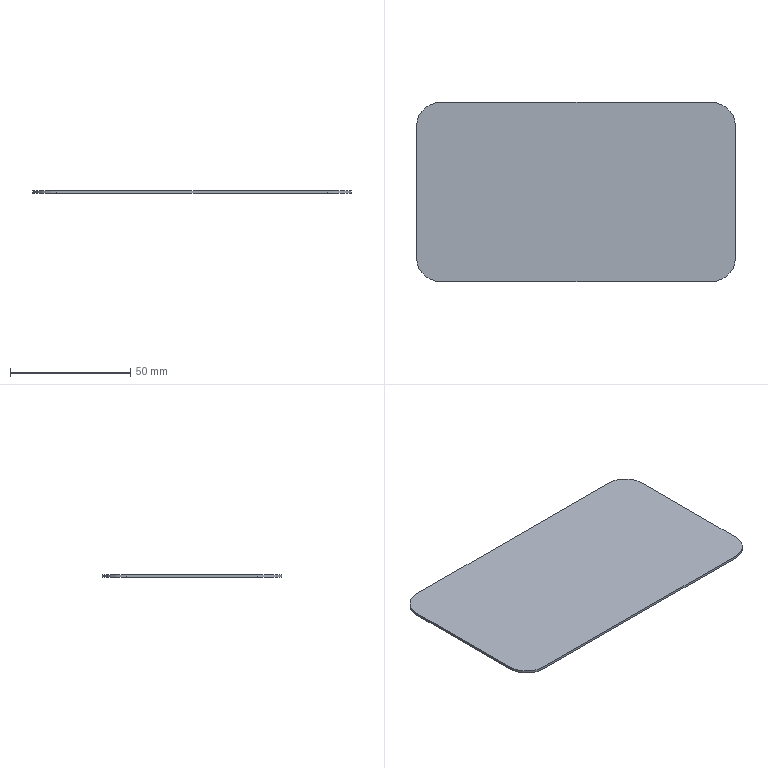Part | SolidWorks | features Extrusion 1, Fillet 1 | 1 solid | 10 faces | box 132.8 x 74.7 x 1 mm | volume 9834 mm3 | plane 6 | cylinder 4 | commonest cylinder face diameters 20 x4
STEP:
#1=CARTESIAN_POINT('',(-66.4,-27.35,1.));
#2=VERTEX_POINT('',#1);
#3=CARTESIAN_POINT('',(-66.4,27.35,1.));
#4=VERTEX_POINT('',#3);
#5=CARTESIAN_POINT('',(-66.4,-37.35,1.));
#6=DIRECTION('',(0.,1.,0.));
#7=VECTOR('',#6,1000.);
#8=LINE('',#5,#7);
#9=EDGE_CURVE('',#2,#4,#8,.T.);
#10=ORIENTED_EDGE('',*,*,#9,.T.);
#11=CARTESIAN_POINT('',(-66.4,27.35,0.));
#12=VERTEX_POINT('',#11);
#13=CARTESIAN_POINT('',(-66.4,27.35,1.));
#14=DIRECTION('',(0.,0.,-1.));
#15=VECTOR('',#14,1000.);
#16=LINE('',#13,#15);
#17=EDGE_CURVE('',#4,#12,#16,.T.);
#18=ORIENTED_EDGE('',*,*,#17,.T.);
#19=CARTESIAN_POINT('',(-66.4,-27.35,0.));
#20=VERTEX_POINT('',#19);
#21=CARTESIAN_POINT('',(-66.4,-37.35,0.));
#22=DIRECTION('',(0.,1.,0.));
#23=VECTOR('',#22,1000.);
#24=LINE('',#21,#23);
#25=EDGE_CURVE('',#20,#12,#24,.T.);
#26=ORIENTED_EDGE('',*,*,#25,.F.);
#27=CARTESIAN_POINT('',(-66.4,-27.35,1.));
#28=DIRECTION('',(0.,0.,1.));
#29=VECTOR('',#28,1000.);
#30=LINE('',#27,#29);
#31=EDGE_CURVE('',#20,#2,#30,.T.);
#32=ORIENTED_EDGE('',*,*,#31,.T.);
#33=EDGE_LOOP('',(#10,#18,#26,#32));
#34=FACE_OUTER_BOUND('',#33,.T.);
#35=CARTESIAN_POINT('',(-66.4,-37.35,1.));
#36=DIRECTION('',(-1.,0.,0.));
#37=DIRECTION('',(0.,0.,1.));
#38=AXIS2_PLACEMENT_3D('',#35,#36,#37);
#39=PLANE('',#38);
#40=ADVANCED_FACE('',(#34),#39,.T.);
#41=CARTESIAN_POINT('',(-56.4,-37.35,0.));
#42=VERTEX_POINT('',#41);
#43=CARTESIAN_POINT('',(56.4,-37.35,0.));
#44=VERTEX_POINT('',#43);
#45=CARTESIAN_POINT('',(-66.4,-37.35,0.));
#46=DIRECTION('',(1.,0.,0.));
#47=VECTOR('',#46,1000.);
#48=LINE('',#45,#47);
#49=EDGE_CURVE('',#42,#44,#48,.T.);
#50=ORIENTED_EDGE('',*,*,#49,.T.);
#51=CARTESIAN_POINT('',(56.4,-37.35,1.));
#52=VERTEX_POINT('',#51);
#53=CARTESIAN_POINT('',(56.4,-37.35,1.));
#54=DIRECTION('',(0.,0.,1.));
#55=VECTOR('',#54,1000.);
#56=LINE('',#53,#55);
#57=EDGE_CURVE('',#44,#52,#56,.T.);
#58=ORIENTED_EDGE('',*,*,#57,.T.);
#59=CARTESIAN_POINT('',(-56.4,-37.35,1.));
#60=VERTEX_POINT('',#59);
#61=CARTESIAN_POINT('',(-66.4,-37.35,1.));
#62=DIRECTION('',(1.,0.,0.));
#63=VECTOR('',#62,1000.);
#64=LINE('',#61,#63);
#65=EDGE_CURVE('',#60,#52,#64,.T.);
#66=ORIENTED_EDGE('',*,*,#65,.F.);
#67=CARTESIAN_POINT('',(-56.4,-37.35,0.));
#68=DIRECTION('',(0.,0.,-1.));
#69=VECTOR('',#68,1000.);
#70=LINE('',#67,#69);
#71=EDGE_CURVE('',#60,#42,#70,.T.);
#72=ORIENTED_EDGE('',*,*,#71,.T.);
#73=EDGE_LOOP('',(#50,#58,#66,#72));
#74=FACE_OUTER_BOUND('',#73,.T.);
#75=CARTESIAN_POINT('',(-66.4,-37.35,1.));
#76=DIRECTION('',(0.,1.,0.));
#77=DIRECTION('',(0.,0.,1.));
#78=AXIS2_PLACEMENT_3D('',#75,#76,#77);
#79=PLANE('',#78);
#80=ADVANCED_FACE('',(#74),#79,.F.);
#81=CARTESIAN_POINT('',(66.4,-27.35,0.));
#82=VERTEX_POINT('',#81);
#83=CARTESIAN_POINT('',(66.4,27.35,0.));
#84=VERTEX_POINT('',#83);
#85=CARTESIAN_POINT('',(66.4,-37.35,0.));
#86=DIRECTION('',(0.,1.,0.));
#87=VECTOR('',#86,1000.);
#88=LINE('',#85,#87);
#89=EDGE_CURVE('',#82,#84,#88,.T.);
#90=ORIENTED_EDGE('',*,*,#89,.T.);
#91=CARTESIAN_POINT('',(66.4,27.35,1.));
#92=VERTEX_POINT('',#91);
#93=CARTESIAN_POINT('',(66.4,27.35,1.));
#94=DIRECTION('',(0.,0.,1.));
#95=VECTOR('',#94,1000.);
#96=LINE('',#93,#95);
#97=EDGE_CURVE('',#84,#92,#96,.T.);
#98=ORIENTED_EDGE('',*,*,#97,.T.);
#99=CARTESIAN_POINT('',(66.4,-27.35,1.));
#100=VERTEX_POINT('',#99);
#101=CARTESIAN_POINT('',(66.4,-37.35,1.));
#102=DIRECTION('',(0.,1.,0.));
#103=VECTOR('',#102,1000.);
#104=LINE('',#101,#103);
#105=EDGE_CURVE('',#100,#92,#104,.T.);
#106=ORIENTED_EDGE('',*,*,#105,.F.);
#107=CARTESIAN_POINT('',(66.4,-27.35,1.));
#108=DIRECTION('',(0.,0.,-1.));
#109=VECTOR('',#108,1000.);
#110=LINE('',#107,#109);
#111=EDGE_CURVE('',#100,#82,#110,.T.);
#112=ORIENTED_EDGE('',*,*,#111,.T.);
#113=EDGE_LOOP('',(#90,#98,#106,#112));
#114=FACE_OUTER_BOUND('',#113,.T.);
#115=CARTESIAN_POINT('',(66.4,-37.35,1.));
#116=DIRECTION('',(-1.,0.,0.));
#117=DIRECTION('',(0.,0.,1.));
#118=AXIS2_PLACEMENT_3D('',#115,#116,#117);
#119=PLANE('',#118);
#120=ADVANCED_FACE('',(#114),#119,.F.);
#121=CARTESIAN_POINT('',(-56.4,37.35,1.));
#122=VERTEX_POINT('',#121);
#123=CARTESIAN_POINT('',(56.4,37.35,1.));
#124=VERTEX_POINT('',#123);
#125=CARTESIAN_POINT('',(-66.4,37.35,1.));
#126=DIRECTION('',(1.,0.,0.));
#127=VECTOR('',#126,1000.);
#128=LINE('',#125,#127);
#129=EDGE_CURVE('',#122,#124,#128,.T.);
#130=ORIENTED_EDGE('',*,*,#129,.T.);
#131=CARTESIAN_POINT('',(56.4,37.35,0.));
#132=VERTEX_POINT('',#131);
#133=CARTESIAN_POINT('',(56.4,37.35,0.));
#134=DIRECTION('',(0.,0.,-1.));
#135=VECTOR('',#134,1000.);
#136=LINE('',#133,#135);
#137=EDGE_CURVE('',#124,#132,#136,.T.);
#138=ORIENTED_EDGE('',*,*,#137,.T.);
#139=CARTESIAN_POINT('',(-56.4,37.35,0.));
#140=VERTEX_POINT('',#139);
#141=CARTESIAN_POINT('',(-66.4,37.35,0.));
#142=DIRECTION('',(1.,0.,0.));
#143=VECTOR('',#142,1000.);
#144=LINE('',#141,#143);
#145=EDGE_CURVE('',#140,#132,#144,.T.);
#146=ORIENTED_EDGE('',*,*,#145,.F.);
#147=CARTESIAN_POINT('',(-56.4,37.35,1.));
#148=DIRECTION('',(0.,0.,1.));
#149=VECTOR('',#148,1000.);
#150=LINE('',#147,#149);
#151=EDGE_CURVE('',#140,#122,#150,.T.);
#152=ORIENTED_EDGE('',*,*,#151,.T.);
#153=EDGE_LOOP('',(#130,#138,#146,#152));
#154=FACE_OUTER_BOUND('',#153,.T.);
#155=CARTESIAN_POINT('',(-66.4,37.35,1.));
#156=DIRECTION('',(0.,1.,0.));
#157=DIRECTION('',(0.,0.,1.));
#158=AXIS2_PLACEMENT_3D('',#155,#156,#157);
#159=PLANE('',#158);
#160=ADVANCED_FACE('',(#154),#159,.T.);
#161=ORIENTED_EDGE('',*,*,#105,.T.);
#162=CARTESIAN_POINT('',(56.4,27.35,1.));
#163=DIRECTION('',(0.,0.,1.));
#164=DIRECTION('',(-1.,0.,0.));
#165=AXIS2_PLACEMENT_3D('',#162,#163,#164);
#166=CIRCLE('',#165,10.);
#167=EDGE_CURVE('',#92,#124,#166,.T.);
#168=ORIENTED_EDGE('',*,*,#167,.T.);
#169=ORIENTED_EDGE('',*,*,#129,.F.);
#170=CARTESIAN_POINT('',(-56.4,27.35,1.));
#171=DIRECTION('',(0.,0.,1.));
#172=DIRECTION('',(-1.,0.,0.));
#173=AXIS2_PLACEMENT_3D('',#170,#171,#172);
#174=CIRCLE('',#173,10.);
#175=EDGE_CURVE('',#122,#4,#174,.T.);
#176=ORIENTED_EDGE('',*,*,#175,.T.);
#177=ORIENTED_EDGE('',*,*,#9,.F.);
#178=CARTESIAN_POINT('',(-56.4,-27.35,1.));
#179=DIRECTION('',(0.,0.,1.));
#180=DIRECTION('',(-1.,0.,0.));
#181=AXIS2_PLACEMENT_3D('',#178,#179,#180);
#182=CIRCLE('',#181,10.);
#183=EDGE_CURVE('',#2,#60,#182,.T.);
#184=ORIENTED_EDGE('',*,*,#183,.T.);
#185=ORIENTED_EDGE('',*,*,#65,.T.);
#186=CARTESIAN_POINT('',(56.4,-27.35,1.));
#187=DIRECTION('',(0.,0.,1.));
#188=DIRECTION('',(-1.,0.,0.));
#189=AXIS2_PLACEMENT_3D('',#186,#187,#188);
#190=CIRCLE('',#189,10.);
#191=EDGE_CURVE('',#52,#100,#190,.T.);
#192=ORIENTED_EDGE('',*,*,#191,.T.);
#193=EDGE_LOOP('',(#161,#168,#169,#176,#177,#184,#185,#192));
#194=FACE_OUTER_BOUND('',#193,.T.);
#195=CARTESIAN_POINT('',(0.,0.,1.));
#196=DIRECTION('',(0.,0.,-1.));
#197=DIRECTION('',(-1.,0.,0.));
#198=AXIS2_PLACEMENT_3D('',#195,#196,#197);
#199=PLANE('',#198);
#200=ADVANCED_FACE('',(#194),#199,.F.);
#201=ORIENTED_EDGE('',*,*,#145,.T.);
#202=CARTESIAN_POINT('',(56.4,27.35,0.));
#203=DIRECTION('',(0.,0.,-1.));
#204=DIRECTION('',(-1.,0.,0.));
#205=AXIS2_PLACEMENT_3D('',#202,#203,#204);
#206=CIRCLE('',#205,10.);
#207=EDGE_CURVE('',#132,#84,#206,.T.);
#208=ORIENTED_EDGE('',*,*,#207,.T.);
#209=ORIENTED_EDGE('',*,*,#89,.F.);
#210=CARTESIAN_POINT('',(56.4,-27.35,0.));
#211=DIRECTION('',(0.,0.,-1.));
#212=DIRECTION('',(-1.,0.,0.));
#213=AXIS2_PLACEMENT_3D('',#210,#211,#212);
#214=CIRCLE('',#213,10.);
#215=EDGE_CURVE('',#82,#44,#214,.T.);
#216=ORIENTED_EDGE('',*,*,#215,.T.);
#217=ORIENTED_EDGE('',*,*,#49,.F.);
#218=CARTESIAN_POINT('',(-56.4,-27.35,0.));
#219=DIRECTION('',(0.,0.,-1.));
#220=DIRECTION('',(-1.,0.,0.));
#221=AXIS2_PLACEMENT_3D('',#218,#219,#220);
#222=CIRCLE('',#221,10.);
#223=EDGE_CURVE('',#42,#20,#222,.T.);
#224=ORIENTED_EDGE('',*,*,#223,.T.);
#225=ORIENTED_EDGE('',*,*,#25,.T.);
#226=CARTESIAN_POINT('',(-56.4,27.35,0.));
#227=DIRECTION('',(0.,0.,-1.));
#228=DIRECTION('',(-1.,0.,0.));
#229=AXIS2_PLACEMENT_3D('',#226,#227,#228);
#230=CIRCLE('',#229,10.);
#231=EDGE_CURVE('',#12,#140,#230,.T.);
#232=ORIENTED_EDGE('',*,*,#231,.T.);
#233=EDGE_LOOP('',(#201,#208,#209,#216,#217,#224,#225,#232));
#234=FACE_OUTER_BOUND('',#233,.T.);
#235=CARTESIAN_POINT('',(0.,0.,0.));
#236=DIRECTION('',(0.,0.,-1.));
#237=DIRECTION('',(-1.,0.,0.));
#238=AXIS2_PLACEMENT_3D('',#235,#236,#237);
#239=PLANE('',#238);
#240=ADVANCED_FACE('',(#234),#239,.T.);
#241=ORIENTED_EDGE('',*,*,#167,.F.);
#242=ORIENTED_EDGE('',*,*,#97,.F.);
#243=ORIENTED_EDGE('',*,*,#207,.F.);
#244=ORIENTED_EDGE('',*,*,#137,.F.);
#245=EDGE_LOOP('',(#241,#242,#243,#244));
#246=FACE_OUTER_BOUND('',#245,.T.);
#247=CARTESIAN_POINT('',(56.4,27.35,1.));
#248=DIRECTION('',(0.,0.,1.));
#249=DIRECTION('',(1.,0.,0.));
#250=AXIS2_PLACEMENT_3D('',#247,#248,#249);
#251=CYLINDRICAL_SURFACE('',#250,10.);
#252=ADVANCED_FACE('',(#246),#251,.T.);
#253=ORIENTED_EDGE('',*,*,#191,.F.);
#254=ORIENTED_EDGE('',*,*,#57,.F.);
#255=ORIENTED_EDGE('',*,*,#215,.F.);
#256=ORIENTED_EDGE('',*,*,#111,.F.);
#257=EDGE_LOOP('',(#253,#254,#255,#256));
#258=FACE_OUTER_BOUND('',#257,.T.);
#259=CARTESIAN_POINT('',(56.4,-27.35,1.));
#260=DIRECTION('',(0.,0.,-1.));
#261=DIRECTION('',(-1.,0.,0.));
#262=AXIS2_PLACEMENT_3D('',#259,#260,#261);
#263=CYLINDRICAL_SURFACE('',#262,10.);
#264=ADVANCED_FACE('',(#258),#263,.T.);
#265=ORIENTED_EDGE('',*,*,#175,.F.);
#266=ORIENTED_EDGE('',*,*,#151,.F.);
#267=ORIENTED_EDGE('',*,*,#231,.F.);
#268=ORIENTED_EDGE('',*,*,#17,.F.);
#269=EDGE_LOOP('',(#265,#266,#267,#268));
#270=FACE_OUTER_BOUND('',#269,.T.);
#271=CARTESIAN_POINT('',(-56.4,27.35,1.));
#272=DIRECTION('',(0.,0.,-1.));
#273=DIRECTION('',(-1.,0.,0.));
#274=AXIS2_PLACEMENT_3D('',#271,#272,#273);
#275=CYLINDRICAL_SURFACE('',#274,10.);
#276=ADVANCED_FACE('',(#270),#275,.T.);
#277=ORIENTED_EDGE('',*,*,#183,.F.);
#278=ORIENTED_EDGE('',*,*,#31,.F.);
#279=ORIENTED_EDGE('',*,*,#223,.F.);
#280=ORIENTED_EDGE('',*,*,#71,.F.);
#281=EDGE_LOOP('',(#277,#278,#279,#280));
#282=FACE_OUTER_BOUND('',#281,.T.);
#283=CARTESIAN_POINT('',(-56.4,-27.35,1.));
#284=DIRECTION('',(0.,0.,1.));
#285=DIRECTION('',(1.,0.,0.));
#286=AXIS2_PLACEMENT_3D('',#283,#284,#285);
#287=CYLINDRICAL_SURFACE('',#286,10.);
#288=ADVANCED_FACE('',(#282),#287,.T.);
#289=CLOSED_SHELL('',(#40,#80,#120,#160,#200,#240,#252,#264,#276,#288));
#290=MANIFOLD_SOLID_BREP('',#289);
#291=CARTESIAN_POINT('',(0.,0.,0.));
#292=DIRECTION('',(0.,0.,1.));
#293=DIRECTION('',(1.,0.,0.));
#294=AXIS2_PLACEMENT_3D('',#291,#292,#293);
#295=(LENGTH_UNIT()NAMED_UNIT(*)SI_UNIT(.MILLI.,.METRE.));
#296=UNCERTAINTY_MEASURE_WITH_UNIT(LENGTH_MEASURE(0.00001),#295,'','');
#297=(NAMED_UNIT(*)PLANE_ANGLE_UNIT()SI_UNIT($,.RADIAN.));
#298=(NAMED_UNIT(*)SI_UNIT($,.STERADIAN.)SOLID_ANGLE_UNIT());
#299=(GEOMETRIC_REPRESENTATION_CONTEXT(3)GLOBAL_UNCERTAINTY_ASSIGNED_CONTEXT((#296))GLOBAL_UNIT_ASSIGNED_CONTEXT((#295,#297,#298))REPRESENTATION_CONTEXT('',''));
#300=ADVANCED_BREP_SHAPE_REPRESENTATION('',(#290,#294),#299);